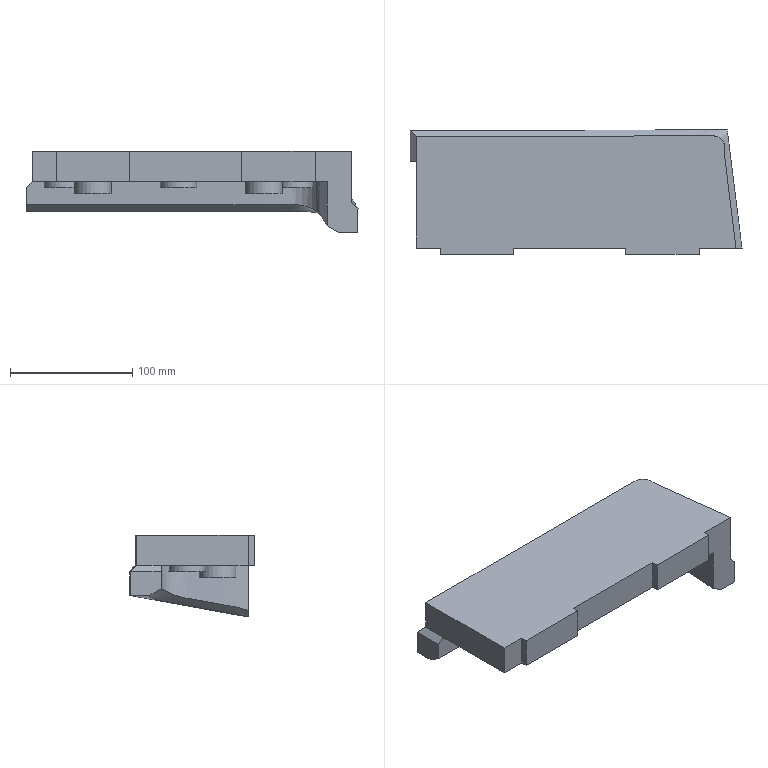Part | NX | features solid 2 | 1 solid | 32 faces | box 272.021 x 101.925 x 67.461 mm | volume 860877 mm3 | plane 20 | spline 7 | cylinder 5 | commonest cylinder face diameters 30 x5